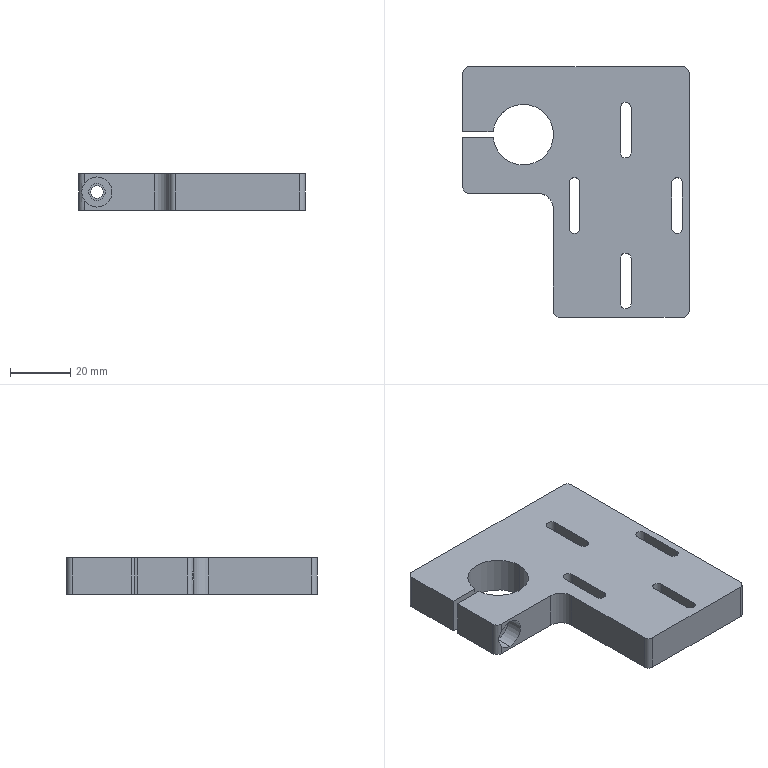Part | SolidWorks | features ICE 4, HoleWzd 3, Fillet 2, LPattern 2, Extrusion 1, MoveFace 1 | 1 solid | 42 faces | box 75 x 83 x 12 mm | volume 51875 mm3 | cylinder 22 | plane 20 | commonest cylinder face diameters 3.5 x8 4 x5 10 x3 4.2 x2 5.5 x2 20.1 x2
STEP:
#1=CARTESIAN_POINT('',(-31.5,40.,2.1));
#2=VERTEX_POINT('',#1);
#3=CARTESIAN_POINT('',(-31.5,40.,-2.1));
#4=VERTEX_POINT('',#3);
#5=CARTESIAN_POINT('',(-31.5,40.,0.));
#6=DIRECTION('',(0.,-1.,0.));
#7=DIRECTION('',(1.,0.,0.));
#8=AXIS2_PLACEMENT_3D('',#5,#6,#7);
#9=CIRCLE('',#8,2.1);
#10=EDGE_CURVE('',#2,#4,#9,.T.);
#11=ORIENTED_EDGE('',*,*,#10,.F.);
#12=CARTESIAN_POINT('',(-31.5,18.5,2.1));
#13=VERTEX_POINT('',#12);
#14=CARTESIAN_POINT('',(-31.5,18.5,2.1));
#15=DIRECTION('',(0.,-1.,0.));
#16=VECTOR('',#15,1000.);
#17=LINE('',#14,#16);
#18=EDGE_CURVE('',#2,#13,#17,.T.);
#19=ORIENTED_EDGE('',*,*,#18,.T.);
#20=CARTESIAN_POINT('',(-31.5,18.5,-2.1));
#21=VERTEX_POINT('',#20);
#22=CARTESIAN_POINT('',(-31.5,18.5,0.));
#23=DIRECTION('',(0.,-1.,0.));
#24=DIRECTION('',(0.,0.,-1.));
#25=AXIS2_PLACEMENT_3D('',#22,#23,#24);
#26=CIRCLE('',#25,2.1);
#27=EDGE_CURVE('',#13,#21,#26,.T.);
#28=ORIENTED_EDGE('',*,*,#27,.T.);
#29=CARTESIAN_POINT('',(-31.5,18.5,-2.1));
#30=DIRECTION('',(0.,-1.,0.));
#31=VECTOR('',#30,1000.);
#32=LINE('',#29,#31);
#33=EDGE_CURVE('',#4,#21,#32,.T.);
#34=ORIENTED_EDGE('',*,*,#33,.F.);
#35=EDGE_LOOP('',(#11,#19,#28,#34));
#36=FACE_OUTER_BOUND('',#35,.T.);
#37=CARTESIAN_POINT('',(-31.5,18.5,0.));
#38=DIRECTION('',(0.,-1.,0.));
#39=DIRECTION('',(0.,0.,-1.));
#40=AXIS2_PLACEMENT_3D('',#37,#38,#39);
#41=CYLINDRICAL_SURFACE('',#40,2.1);
#42=ADVANCED_FACE('',(#36),#41,.F.);
#43=CARTESIAN_POINT('',(-31.5,3.7,5.));
#44=VERTEX_POINT('',#43);
#45=CARTESIAN_POINT('',(-31.5,3.7,-5.));
#46=VERTEX_POINT('',#45);
#47=CARTESIAN_POINT('',(-31.5,3.7,0.));
#48=DIRECTION('',(0.,-1.,0.));
#49=DIRECTION('',(0.,0.,-1.));
#50=AXIS2_PLACEMENT_3D('',#47,#48,#49);
#51=CIRCLE('',#50,5.);
#52=EDGE_CURVE('',#44,#46,#51,.T.);
#53=ORIENTED_EDGE('',*,*,#52,.F.);
#54=CARTESIAN_POINT('',(-31.5,-2.,5.));
#55=VERTEX_POINT('',#54);
#56=CARTESIAN_POINT('',(-31.5,-2.,5.));
#57=DIRECTION('',(0.,-1.,0.));
#58=VECTOR('',#57,1000.);
#59=LINE('',#56,#58);
#60=EDGE_CURVE('',#44,#55,#59,.T.);
#61=ORIENTED_EDGE('',*,*,#60,.T.);
#62=CARTESIAN_POINT('',(-35.5,-2.,3.));
#63=VERTEX_POINT('',#62);
#64=CARTESIAN_POINT('',(-31.5,-2.,0.));
#65=DIRECTION('',(0.,-1.,0.));
#66=DIRECTION('',(0.,0.,-1.));
#67=AXIS2_PLACEMENT_3D('',#64,#65,#66);
#68=CIRCLE('',#67,5.);
#69=EDGE_CURVE('',#55,#63,#68,.T.);
#70=ORIENTED_EDGE('',*,*,#69,.T.);
#71=CARTESIAN_POINT('',(-35.5,-2.,-3.));
#72=VERTEX_POINT('',#71);
#73=CARTESIAN_POINT('',(-35.5,-2.,3.));
#74=CARTESIAN_POINT('',(-35.663,-2.,2.782));
#75=CARTESIAN_POINT('',(-35.806,-1.981,2.555));
#76=CARTESIAN_POINT('',(-36.054,-1.926,2.082));
#77=CARTESIAN_POINT('',(-36.159,-1.891,1.835));
#78=CARTESIAN_POINT('',(-36.328,-1.823,1.326));
#79=CARTESIAN_POINT('',(-36.392,-1.791,1.067));
#80=CARTESIAN_POINT('',(-36.478,-1.745,0.5398));
#81=CARTESIAN_POINT('',(-36.5,-1.732,0.2681));
#82=CARTESIAN_POINT('',(-36.5,-1.732,-0.271));
#83=CARTESIAN_POINT('',(-36.478,-1.745,-0.5373));
#84=CARTESIAN_POINT('',(-36.393,-1.79,-1.064));
#85=CARTESIAN_POINT('',(-36.328,-1.823,-1.326));
#86=CARTESIAN_POINT('',(-36.159,-1.89,-1.834));
#87=CARTESIAN_POINT('',(-36.055,-1.926,-2.079));
#88=CARTESIAN_POINT('',(-35.808,-1.98,-2.552));
#89=CARTESIAN_POINT('',(-35.663,-2.,-2.783));
#90=CARTESIAN_POINT('',(-35.5,-2.,-3.));
#91=B_SPLINE_CURVE_WITH_KNOTS('',3,(#73,#74,#75,#76,#77,#78,#79,#80,#81,#82,#83,#84,#85,#86,#87,#88,#89,#90),.UNSPECIFIED.,.F.,.F.,(4,2,2,2,2,2,2,2,4),(0.,0.0008047,0.001609,0.002414,0.003219,0.004024,0.004828,0.005633,0.006438),.UNSPECIFIED.);
#92=EDGE_CURVE('',#63,#72,#91,.T.);
#93=ORIENTED_EDGE('',*,*,#92,.T.);
#94=CARTESIAN_POINT('',(-31.5,-2.,-5.));
#95=VERTEX_POINT('',#94);
#96=CARTESIAN_POINT('',(-31.5,-2.,0.));
#97=DIRECTION('',(0.,-1.,0.));
#98=DIRECTION('',(0.,0.,-1.));
#99=AXIS2_PLACEMENT_3D('',#96,#97,#98);
#100=CIRCLE('',#99,5.);
#101=EDGE_CURVE('',#72,#95,#100,.T.);
#102=ORIENTED_EDGE('',*,*,#101,.T.);
#103=CARTESIAN_POINT('',(-31.5,-2.,-5.));
#104=DIRECTION('',(0.,-1.,0.));
#105=VECTOR('',#104,1000.);
#106=LINE('',#103,#105);
#107=EDGE_CURVE('',#46,#95,#106,.T.);
#108=ORIENTED_EDGE('',*,*,#107,.F.);
#109=EDGE_LOOP('',(#53,#61,#70,#93,#102,#108));
#110=FACE_OUTER_BOUND('',#109,.T.);
#111=CARTESIAN_POINT('',(-31.5,-2.,0.));
#112=DIRECTION('',(0.,-1.,0.));
#113=DIRECTION('',(0.,0.,-1.));
#114=AXIS2_PLACEMENT_3D('',#111,#112,#113);
#115=CYLINDRICAL_SURFACE('',#114,5.);
#116=ADVANCED_FACE('',(#110),#115,.F.);
#117=CARTESIAN_POINT('',(-31.5,16.5,2.75));
#118=VERTEX_POINT('',#117);
#119=CARTESIAN_POINT('',(-31.5,16.5,-2.75));
#120=VERTEX_POINT('',#119);
#121=CARTESIAN_POINT('',(-31.5,16.5,0.));
#122=DIRECTION('',(0.,-1.,0.));
#123=DIRECTION('',(1.,0.,0.));
#124=AXIS2_PLACEMENT_3D('',#121,#122,#123);
#125=CIRCLE('',#124,2.75);
#126=EDGE_CURVE('',#118,#120,#125,.T.);
#127=ORIENTED_EDGE('',*,*,#126,.F.);
#128=CARTESIAN_POINT('',(-31.5,3.7,2.75));
#129=VERTEX_POINT('',#128);
#130=CARTESIAN_POINT('',(-31.5,-2.,2.75));
#131=DIRECTION('',(0.,-1.,0.));
#132=VECTOR('',#131,1000.);
#133=LINE('',#130,#132);
#134=EDGE_CURVE('',#118,#129,#133,.T.);
#135=ORIENTED_EDGE('',*,*,#134,.T.);
#136=CARTESIAN_POINT('',(-31.5,3.7,-2.75));
#137=VERTEX_POINT('',#136);
#138=CARTESIAN_POINT('',(-31.5,3.7,0.));
#139=DIRECTION('',(0.,-1.,0.));
#140=DIRECTION('',(0.,0.,-1.));
#141=AXIS2_PLACEMENT_3D('',#138,#139,#140);
#142=CIRCLE('',#141,2.75);
#143=EDGE_CURVE('',#129,#137,#142,.T.);
#144=ORIENTED_EDGE('',*,*,#143,.T.);
#145=CARTESIAN_POINT('',(-31.5,-2.,-2.75));
#146=DIRECTION('',(0.,-1.,0.));
#147=VECTOR('',#146,1000.);
#148=LINE('',#145,#147);
#149=EDGE_CURVE('',#120,#137,#148,.T.);
#150=ORIENTED_EDGE('',*,*,#149,.F.);
#151=EDGE_LOOP('',(#127,#135,#144,#150));
#152=FACE_OUTER_BOUND('',#151,.T.);
#153=CARTESIAN_POINT('',(-31.5,-2.,0.));
#154=DIRECTION('',(0.,-1.,0.));
#155=DIRECTION('',(0.,0.,-1.));
#156=AXIS2_PLACEMENT_3D('',#153,#154,#155);
#157=CYLINDRICAL_SURFACE('',#156,2.75);
#158=ADVANCED_FACE('',(#152),#157,.F.);
#159=CARTESIAN_POINT('',(-27.5,18.5,-6.));
#160=VERTEX_POINT('',#159);
#161=CARTESIAN_POINT('',(-7.45,17.5,-6.));
#162=VERTEX_POINT('',#161);
#163=CARTESIAN_POINT('',(-17.5,17.5,-6.));
#164=DIRECTION('',(0.,0.,-1.));
#165=DIRECTION('',(1.,0.,0.));
#166=AXIS2_PLACEMENT_3D('',#163,#164,#165);
#167=CIRCLE('',#166,10.05);
#168=EDGE_CURVE('',#160,#162,#167,.T.);
#169=ORIENTED_EDGE('',*,*,#168,.T.);
#170=CARTESIAN_POINT('',(-7.45,17.5,6.));
#171=VERTEX_POINT('',#170);
#172=CARTESIAN_POINT('',(-7.45,17.5,-6.001));
#173=DIRECTION('',(0.,0.,1.));
#174=VECTOR('',#173,1000.);
#175=LINE('',#172,#174);
#176=EDGE_CURVE('',#162,#171,#175,.T.);
#177=ORIENTED_EDGE('',*,*,#176,.T.);
#178=CARTESIAN_POINT('',(-27.5,18.5,6.));
#179=VERTEX_POINT('',#178);
#180=CARTESIAN_POINT('',(-17.5,17.5,6.));
#181=DIRECTION('',(0.,0.,1.));
#182=DIRECTION('',(1.,0.,0.));
#183=AXIS2_PLACEMENT_3D('',#180,#181,#182);
#184=CIRCLE('',#183,10.05);
#185=EDGE_CURVE('',#171,#179,#184,.T.);
#186=ORIENTED_EDGE('',*,*,#185,.T.);
#187=CARTESIAN_POINT('',(-27.5,18.5,-6.001));
#188=DIRECTION('',(0.,0.,1.));
#189=VECTOR('',#188,1000.);
#190=LINE('',#187,#189);
#191=EDGE_CURVE('',#160,#179,#190,.T.);
#192=ORIENTED_EDGE('',*,*,#191,.F.);
#193=EDGE_LOOP('',(#169,#177,#186,#192));
#194=FACE_OUTER_BOUND('',#193,.T.);
#195=CARTESIAN_POINT('',(-17.5,17.5,-6.001));
#196=DIRECTION('',(0.,0.,1.));
#197=DIRECTION('',(1.,0.,0.));
#198=AXIS2_PLACEMENT_3D('',#195,#196,#197);
#199=CYLINDRICAL_SURFACE('',#198,10.05);
#200=ADVANCED_FACE('',(#194),#199,.F.);
#201=ORIENTED_EDGE('',*,*,#101,.F.);
#202=CARTESIAN_POINT('',(-35.5,-2.,-6.));
#203=VERTEX_POINT('',#202);
#204=CARTESIAN_POINT('',(-35.5,-2.,6.001));
#205=DIRECTION('',(0.,0.,-1.));
#206=VECTOR('',#205,1000.);
#207=LINE('',#204,#206);
#208=EDGE_CURVE('',#72,#203,#207,.T.);
#209=ORIENTED_EDGE('',*,*,#208,.T.);
#210=CARTESIAN_POINT('',(-12.5,-2.,-6.));
#211=VERTEX_POINT('',#210);
#212=CARTESIAN_POINT('',(-37.5,-2.,-6.));
#213=DIRECTION('',(1.,0.,0.));
#214=VECTOR('',#213,1000.);
#215=LINE('',#212,#214);
#216=EDGE_CURVE('',#203,#211,#215,.T.);
#217=ORIENTED_EDGE('',*,*,#216,.T.);
#218=CARTESIAN_POINT('',(-12.5,-2.,6.));
#219=VERTEX_POINT('',#218);
#220=CARTESIAN_POINT('',(-12.5,-2.,6.));
#221=DIRECTION('',(0.,0.,1.));
#222=VECTOR('',#221,1000.);
#223=LINE('',#220,#222);
#224=EDGE_CURVE('',#211,#219,#223,.T.);
#225=ORIENTED_EDGE('',*,*,#224,.T.);
#226=CARTESIAN_POINT('',(-35.5,-2.,6.));
#227=VERTEX_POINT('',#226);
#228=CARTESIAN_POINT('',(-37.5,-2.,6.));
#229=DIRECTION('',(1.,0.,0.));
#230=VECTOR('',#229,1000.);
#231=LINE('',#228,#230);
#232=EDGE_CURVE('',#227,#219,#231,.T.);
#233=ORIENTED_EDGE('',*,*,#232,.F.);
#234=CARTESIAN_POINT('',(-35.5,-2.,6.001));
#235=DIRECTION('',(0.,0.,-1.));
#236=VECTOR('',#235,1000.);
#237=LINE('',#234,#236);
#238=EDGE_CURVE('',#227,#63,#237,.T.);
#239=ORIENTED_EDGE('',*,*,#238,.T.);
#240=ORIENTED_EDGE('',*,*,#69,.F.);
#241=CARTESIAN_POINT('',(-31.5,-2.,0.));
#242=DIRECTION('',(0.,-1.,0.));
#243=DIRECTION('',(0.,0.,-1.));
#244=AXIS2_PLACEMENT_3D('',#241,#242,#243);
#245=CIRCLE('',#244,5.);
#246=EDGE_CURVE('',#95,#55,#245,.T.);
#247=ORIENTED_EDGE('',*,*,#246,.F.);
#248=EDGE_LOOP('',(#201,#209,#217,#225,#233,#239,#240,#247));
#249=FACE_OUTER_BOUND('',#248,.T.);
#250=CARTESIAN_POINT('',(-37.5,-2.,6.001));
#251=DIRECTION('',(0.,1.,0.));
#252=DIRECTION('',(-1.,0.,0.));
#253=AXIS2_PLACEMENT_3D('',#250,#251,#252);
#254=PLANE('',#253);
#255=ADVANCED_FACE('',(#249),#254,.F.);
#256=CARTESIAN_POINT('',(31.75,-13.5,-6.));
#257=VERTEX_POINT('',#256);
#258=CARTESIAN_POINT('',(31.75,1.5,-6.));
#259=VERTEX_POINT('',#258);
#260=CARTESIAN_POINT('',(31.75,-13.5,-6.));
#261=DIRECTION('',(0.,1.,0.));
#262=VECTOR('',#261,1000.);
#263=LINE('',#260,#262);
#264=EDGE_CURVE('',#257,#259,#263,.T.);
#265=ORIENTED_EDGE('',*,*,#264,.F.);
#266=CARTESIAN_POINT('',(35.25,-13.5,-6.));
#267=VERTEX_POINT('',#266);
#268=CARTESIAN_POINT('',(33.5,-13.5,-6.));
#269=DIRECTION('',(0.,0.,-1.));
#270=DIRECTION('',(-1.,0.,0.));
#271=AXIS2_PLACEMENT_3D('',#268,#269,#270);
#272=CIRCLE('',#271,1.75);
#273=EDGE_CURVE('',#267,#257,#272,.T.);
#274=ORIENTED_EDGE('',*,*,#273,.F.);
#275=CARTESIAN_POINT('',(35.25,1.5,-6.));
#276=VERTEX_POINT('',#275);
#277=CARTESIAN_POINT('',(35.25,-13.5,-6.));
#278=DIRECTION('',(0.,-1.,0.));
#279=VECTOR('',#278,1000.);
#280=LINE('',#277,#279);
#281=EDGE_CURVE('',#276,#267,#280,.T.);
#282=ORIENTED_EDGE('',*,*,#281,.F.);
#283=CARTESIAN_POINT('',(33.5,1.5,-6.));
#284=DIRECTION('',(0.,0.,-1.));
#285=DIRECTION('',(-1.,0.,0.));
#286=AXIS2_PLACEMENT_3D('',#283,#284,#285);
#287=CIRCLE('',#286,1.75);
#288=EDGE_CURVE('',#259,#276,#287,.T.);
#289=ORIENTED_EDGE('',*,*,#288,.F.);
#290=EDGE_LOOP('',(#265,#274,#282,#289));
#291=FACE_BOUND('',#290,.T.);
#292=CARTESIAN_POINT('',(14.75,-38.5,-6.));
#293=VERTEX_POINT('',#292);
#294=CARTESIAN_POINT('',(14.75,-23.5,-6.));
#295=VERTEX_POINT('',#294);
#296=CARTESIAN_POINT('',(14.75,-38.5,-6.));
#297=DIRECTION('',(0.,1.,0.));
#298=VECTOR('',#297,1000.);
#299=LINE('',#296,#298);
#300=EDGE_CURVE('',#293,#295,#299,.T.);
#301=ORIENTED_EDGE('',*,*,#300,.F.);
#302=CARTESIAN_POINT('',(18.25,-38.5,-6.));
#303=VERTEX_POINT('',#302);
#304=CARTESIAN_POINT('',(16.5,-38.5,-6.));
#305=DIRECTION('',(0.,0.,-1.));
#306=DIRECTION('',(-1.,0.,0.));
#307=AXIS2_PLACEMENT_3D('',#304,#305,#306);
#308=CIRCLE('',#307,1.75);
#309=EDGE_CURVE('',#303,#293,#308,.T.);
#310=ORIENTED_EDGE('',*,*,#309,.F.);
#311=CARTESIAN_POINT('',(18.25,-23.5,-6.));
#312=VERTEX_POINT('',#311);
#313=CARTESIAN_POINT('',(18.25,-38.5,-6.));
#314=DIRECTION('',(0.,-1.,0.));
#315=VECTOR('',#314,1000.);
#316=LINE('',#313,#315);
#317=EDGE_CURVE('',#312,#303,#316,.T.);
#318=ORIENTED_EDGE('',*,*,#317,.F.);
#319=CARTESIAN_POINT('',(16.5,-23.5,-6.));
#320=DIRECTION('',(0.,0.,-1.));
#321=DIRECTION('',(-1.,0.,0.));
#322=AXIS2_PLACEMENT_3D('',#319,#320,#321);
#323=CIRCLE('',#322,1.75);
#324=EDGE_CURVE('',#295,#312,#323,.T.);
#325=ORIENTED_EDGE('',*,*,#324,.F.);
#326=EDGE_LOOP('',(#301,#310,#318,#325));
#327=FACE_BOUND('',#326,.T.);
#328=CARTESIAN_POINT('',(-2.25,-13.5,-6.));
#329=VERTEX_POINT('',#328);
#330=CARTESIAN_POINT('',(-2.25,1.5,-6.));
#331=VERTEX_POINT('',#330);
#332=CARTESIAN_POINT('',(-2.25,-13.5,-6.));
#333=DIRECTION('',(0.,1.,0.));
#334=VECTOR('',#333,1000.);
#335=LINE('',#332,#334);
#336=EDGE_CURVE('',#329,#331,#335,.T.);
#337=ORIENTED_EDGE('',*,*,#336,.F.);
#338=CARTESIAN_POINT('',(1.25,-13.5,-6.));
#339=VERTEX_POINT('',#338);
#340=CARTESIAN_POINT('',(-0.5,-13.5,-6.));
#341=DIRECTION('',(0.,0.,-1.));
#342=DIRECTION('',(-1.,0.,0.));
#343=AXIS2_PLACEMENT_3D('',#340,#341,#342);
#344=CIRCLE('',#343,1.75);
#345=EDGE_CURVE('',#339,#329,#344,.T.);
#346=ORIENTED_EDGE('',*,*,#345,.F.);
#347=CARTESIAN_POINT('',(1.25,1.5,-6.));
#348=VERTEX_POINT('',#347);
#349=CARTESIAN_POINT('',(1.25,-13.5,-6.));
#350=DIRECTION('',(0.,-1.,0.));
#351=VECTOR('',#350,1000.);
#352=LINE('',#349,#351);
#353=EDGE_CURVE('',#348,#339,#352,.T.);
#354=ORIENTED_EDGE('',*,*,#353,.F.);
#355=CARTESIAN_POINT('',(-0.5,1.5,-6.));
#356=DIRECTION('',(0.,0.,-1.));
#357=DIRECTION('',(-1.,0.,0.));
#358=AXIS2_PLACEMENT_3D('',#355,#356,#357);
#359=CIRCLE('',#358,1.75);
#360=EDGE_CURVE('',#331,#348,#359,.T.);
#361=ORIENTED_EDGE('',*,*,#360,.F.);
#362=EDGE_LOOP('',(#337,#346,#354,#361));
#363=FACE_BOUND('',#362,.T.);
#364=CARTESIAN_POINT('',(14.75,11.5,-6.));
#365=VERTEX_POINT('',#364);
#366=CARTESIAN_POINT('',(14.75,26.5,-6.));
#367=VERTEX_POINT('',#366);
#368=CARTESIAN_POINT('',(14.75,11.5,-6.));
#369=DIRECTION('',(0.,1.,0.));
#370=VECTOR('',#369,1000.);
#371=LINE('',#368,#370);
#372=EDGE_CURVE('',#365,#367,#371,.T.);
#373=ORIENTED_EDGE('',*,*,#372,.F.);
#374=CARTESIAN_POINT('',(18.25,11.5,-6.));
#375=VERTEX_POINT('',#374);
#376=CARTESIAN_POINT('',(16.5,11.5,-6.));
#377=DIRECTION('',(0.,0.,-1.));
#378=DIRECTION('',(-1.,0.,0.));
#379=AXIS2_PLACEMENT_3D('',#376,#377,#378);
#380=CIRCLE('',#379,1.75);
#381=EDGE_CURVE('',#375,#365,#380,.T.);
#382=ORIENTED_EDGE('',*,*,#381,.F.);
#383=CARTESIAN_POINT('',(18.25,26.5,-6.));
#384=VERTEX_POINT('',#383);
#385=CARTESIAN_POINT('',(18.25,11.5,-6.));
#386=DIRECTION('',(0.,-1.,0.));
#387=VECTOR('',#386,1000.);
#388=LINE('',#385,#387);
#389=EDGE_CURVE('',#384,#375,#388,.T.);
#390=ORIENTED_EDGE('',*,*,#389,.F.);
#391=CARTESIAN_POINT('',(16.5,26.5,-6.));
#392=DIRECTION('',(0.,0.,-1.));
#393=DIRECTION('',(-1.,0.,0.));
#394=AXIS2_PLACEMENT_3D('',#391,#392,#393);
#395=CIRCLE('',#394,1.75);
#396=EDGE_CURVE('',#367,#384,#395,.T.);
#397=ORIENTED_EDGE('',*,*,#396,.F.);
#398=EDGE_LOOP('',(#373,#382,#390,#397));
#399=FACE_BOUND('',#398,.T.);
#400=CARTESIAN_POINT('',(35.5,40.,-6.));
#401=VERTEX_POINT('',#400);
#402=CARTESIAN_POINT('',(-35.5,40.,-6.));
#403=VERTEX_POINT('',#402);
#404=CARTESIAN_POINT('',(37.5,40.,-6.));
#405=DIRECTION('',(-1.,0.,0.));
#406=VECTOR('',#405,1000.);
#407=LINE('',#404,#406);
#408=EDGE_CURVE('',#401,#403,#407,.T.);
#409=ORIENTED_EDGE('',*,*,#408,.F.);
#410=CARTESIAN_POINT('',(37.5,38.,-6.));
#411=VERTEX_POINT('',#410);
#412=CARTESIAN_POINT('',(35.5,38.,-6.));
#413=DIRECTION('',(0.,0.,-1.));
#414=DIRECTION('',(1.,0.,0.));
#415=AXIS2_PLACEMENT_3D('',#412,#413,#414);
#416=CIRCLE('',#415,2.);
#417=EDGE_CURVE('',#401,#411,#416,.T.);
#418=ORIENTED_EDGE('',*,*,#417,.T.);
#419=CARTESIAN_POINT('',(37.5,-41.,-6.));
#420=VERTEX_POINT('',#419);
#421=CARTESIAN_POINT('',(37.5,-40.,-6.));
#422=DIRECTION('',(0.,1.,0.));
#423=VECTOR('',#422,1000.);
#424=LINE('',#421,#423);
#425=EDGE_CURVE('',#420,#411,#424,.T.);
#426=ORIENTED_EDGE('',*,*,#425,.F.);
#427=CARTESIAN_POINT('',(35.5,-43.,-6.));
#428=VERTEX_POINT('',#427);
#429=CARTESIAN_POINT('',(35.5,-41.,-6.));
#430=DIRECTION('',(0.,0.,-1.));
#431=DIRECTION('',(1.,0.,0.));
#432=AXIS2_PLACEMENT_3D('',#429,#430,#431);
#433=CIRCLE('',#432,2.);
#434=EDGE_CURVE('',#420,#428,#433,.T.);
#435=ORIENTED_EDGE('',*,*,#434,.T.);
#436=CARTESIAN_POINT('',(-5.5,-43.,-6.));
#437=VERTEX_POINT('',#436);
#438=CARTESIAN_POINT('',(37.5,-43.,-6.));
#439=DIRECTION('',(1.,0.,0.));
#440=VECTOR('',#439,1000.);
#441=LINE('',#438,#440);
#442=EDGE_CURVE('',#437,#428,#441,.T.);
#443=ORIENTED_EDGE('',*,*,#442,.F.);
#444=CARTESIAN_POINT('',(-7.5,-41.,-6.));
#445=VERTEX_POINT('',#444);
#446=CARTESIAN_POINT('',(-5.5,-41.,-6.));
#447=DIRECTION('',(0.,0.,-1.));
#448=DIRECTION('',(1.,0.,0.));
#449=AXIS2_PLACEMENT_3D('',#446,#447,#448);
#450=CIRCLE('',#449,2.);
#451=EDGE_CURVE('',#437,#445,#450,.T.);
#452=ORIENTED_EDGE('',*,*,#451,.T.);
#453=CARTESIAN_POINT('',(-7.5,-7.,-6.));
#454=VERTEX_POINT('',#453);
#455=CARTESIAN_POINT('',(-7.5,-2.,-6.));
#456=DIRECTION('',(0.,-1.,0.));
#457=VECTOR('',#456,1000.);
#458=LINE('',#455,#457);
#459=EDGE_CURVE('',#454,#445,#458,.T.);
#460=ORIENTED_EDGE('',*,*,#459,.F.);
#461=CARTESIAN_POINT('',(-12.5,-7.,-6.));
#462=DIRECTION('',(0.,0.,1.));
#463=DIRECTION('',(1.,0.,0.));
#464=AXIS2_PLACEMENT_3D('',#461,#462,#463);
#465=CIRCLE('',#464,5.);
#466=EDGE_CURVE('',#454,#211,#465,.T.);
#467=ORIENTED_EDGE('',*,*,#466,.T.);
#468=ORIENTED_EDGE('',*,*,#216,.F.);
#469=CARTESIAN_POINT('',(-37.5,0.,-6.));
#470=VERTEX_POINT('',#469);
#471=CARTESIAN_POINT('',(-35.5,0.,-6.));
#472=DIRECTION('',(0.,0.,-1.));
#473=DIRECTION('',(1.,0.,0.));
#474=AXIS2_PLACEMENT_3D('',#471,#472,#473);
#475=CIRCLE('',#474,2.);
#476=EDGE_CURVE('',#203,#470,#475,.T.);
#477=ORIENTED_EDGE('',*,*,#476,.T.);
#478=CARTESIAN_POINT('',(-37.5,16.5,-6.));
#479=VERTEX_POINT('',#478);
#480=CARTESIAN_POINT('',(-37.5,-40.,-6.));
#481=DIRECTION('',(0.,-1.,0.));
#482=VECTOR('',#481,1000.);
#483=LINE('',#480,#482);
#484=EDGE_CURVE('',#479,#470,#483,.T.);
#485=ORIENTED_EDGE('',*,*,#484,.F.);
#486=CARTESIAN_POINT('',(-27.5,16.5,-6.));
#487=VERTEX_POINT('',#486);
#488=CARTESIAN_POINT('',(-52.59,16.5,-6.));
#489=DIRECTION('',(-1.,0.,0.));
#490=VECTOR('',#489,1000.);
#491=LINE('',#488,#490);
#492=EDGE_CURVE('',#487,#479,#491,.T.);
#493=ORIENTED_EDGE('',*,*,#492,.F.);
#494=CARTESIAN_POINT('',(-17.5,17.5,-6.));
#495=DIRECTION('',(0.,0.,-1.));
#496=DIRECTION('',(1.,0.,0.));
#497=AXIS2_PLACEMENT_3D('',#494,#495,#496);
#498=CIRCLE('',#497,10.05);
#499=EDGE_CURVE('',#162,#487,#498,.T.);
#500=ORIENTED_EDGE('',*,*,#499,.F.);
#501=ORIENTED_EDGE('',*,*,#168,.F.);
#502=CARTESIAN_POINT('',(-37.5,18.5,-6.));
#503=VERTEX_POINT('',#502);
#504=CARTESIAN_POINT('',(-52.59,18.5,-6.));
#505=DIRECTION('',(1.,0.,0.));
#506=VECTOR('',#505,1000.);
#507=LINE('',#504,#506);
#508=EDGE_CURVE('',#503,#160,#507,.T.);
#509=ORIENTED_EDGE('',*,*,#508,.F.);
#510=CARTESIAN_POINT('',(-37.5,38.,-6.));
#511=VERTEX_POINT('',#510);
#512=CARTESIAN_POINT('',(-37.5,-40.,-6.));
#513=DIRECTION('',(0.,-1.,0.));
#514=VECTOR('',#513,1000.);
#515=LINE('',#512,#514);
#516=EDGE_CURVE('',#511,#503,#515,.T.);
#517=ORIENTED_EDGE('',*,*,#516,.F.);
#518=CARTESIAN_POINT('',(-35.5,38.,-6.));
#519=DIRECTION('',(0.,0.,-1.));
#520=DIRECTION('',(1.,0.,0.));
#521=AXIS2_PLACEMENT_3D('',#518,#519,#520);
#522=CIRCLE('',#521,2.);
#523=EDGE_CURVE('',#511,#403,#522,.T.);
#524=ORIENTED_EDGE('',*,*,#523,.T.);
#525=EDGE_LOOP('',(#409,#418,#426,#435,#443,#452,#460,#467,#468,#477,#485,#493,#500,#501,#509,#517,#524));
#526=FACE_OUTER_BOUND('',#525,.T.);
#527=CARTESIAN_POINT('',(0.,0.,-6.));
#528=DIRECTION('',(0.,0.,1.));
#529=DIRECTION('',(1.,0.,0.));
#530=AXIS2_PLACEMENT_3D('',#527,#528,#529);
#531=PLANE('',#530);
#532=ADVANCED_FACE('',(#291,#327,#363,#399,#526),#531,.F.);
#533=CARTESIAN_POINT('',(-37.5,38.,6.));
#534=VERTEX_POINT('',#533);
#535=CARTESIAN_POINT('',(-37.5,18.5,6.));
#536=VERTEX_POINT('',#535);
#537=CARTESIAN_POINT('',(-37.5,-40.,6.));
#538=DIRECTION('',(0.,-1.,0.));
#539=VECTOR('',#538,1000.);
#540=LINE('',#537,#539);
#541=EDGE_CURVE('',#534,#536,#540,.T.);
#542=ORIENTED_EDGE('',*,*,#541,.F.);
#543=CARTESIAN_POINT('',(-37.5,38.,6.));
#544=DIRECTION('',(0.,0.,-1.));
#545=VECTOR('',#544,1000.);
#546=LINE('',#543,#545);
#547=EDGE_CURVE('',#534,#511,#546,.T.);
#548=ORIENTED_EDGE('',*,*,#547,.T.);
#549=ORIENTED_EDGE('',*,*,#516,.T.);
#550=CARTESIAN_POINT('',(-37.5,18.5,6.001));
#551=DIRECTION('',(0.,0.,-1.));
#552=VECTOR('',#551,1000.);
#553=LINE('',#550,#552);
#554=EDGE_CURVE('',#536,#503,#553,.T.);
#555=ORIENTED_EDGE('',*,*,#554,.F.);
#556=EDGE_LOOP('',(#542,#548,#549,#555));
#557=FACE_OUTER_BOUND('',#556,.T.);
#558=CARTESIAN_POINT('',(-37.5,-40.,6.));
#559=DIRECTION('',(1.,0.,0.));
#560=DIRECTION('',(0.,0.,-1.));
#561=AXIS2_PLACEMENT_3D('',#558,#559,#560);
#562=PLANE('',#561);
#563=ADVANCED_FACE('',(#557),#562,.F.);
#564=ORIENTED_EDGE('',*,*,#484,.T.);
#565=CARTESIAN_POINT('',(-37.5,0.,6.));
#566=VERTEX_POINT('',#565);
#567=CARTESIAN_POINT('',(-37.5,0.,6.));
#568=DIRECTION('',(0.,0.,1.));
#569=VECTOR('',#568,1000.);
#570=LINE('',#567,#569);
#571=EDGE_CURVE('',#470,#566,#570,.T.);
#572=ORIENTED_EDGE('',*,*,#571,.T.);
#573=CARTESIAN_POINT('',(-37.5,16.5,6.));
#574=VERTEX_POINT('',#573);
#575=CARTESIAN_POINT('',(-37.5,-40.,6.));
#576=DIRECTION('',(0.,-1.,0.));
#577=VECTOR('',#576,1000.);
#578=LINE('',#575,#577);
#579=EDGE_CURVE('',#574,#566,#578,.T.);
#580=ORIENTED_EDGE('',*,*,#579,.F.);
#581=CARTESIAN_POINT('',(-37.5,16.5,6.001));
#582=DIRECTION('',(0.,0.,1.));
#583=VECTOR('',#582,1000.);
#584=LINE('',#581,#583);
#585=EDGE_CURVE('',#479,#574,#584,.T.);
#586=ORIENTED_EDGE('',*,*,#585,.F.);
#587=EDGE_LOOP('',(#564,#572,#580,#586));
#588=FACE_OUTER_BOUND('',#587,.T.);
#589=CARTESIAN_POINT('',(-37.5,-40.,6.));
#590=DIRECTION('',(1.,0.,0.));
#591=DIRECTION('',(0.,0.,-1.));
#592=AXIS2_PLACEMENT_3D('',#589,#590,#591);
#593=PLANE('',#592);
#594=ADVANCED_FACE('',(#588),#593,.F.);
#595=ORIENTED_EDGE('',*,*,#442,.T.);
#596=CARTESIAN_POINT('',(35.5,-43.,6.));
#597=VERTEX_POINT('',#596);
#598=CARTESIAN_POINT('',(35.5,-43.,6.));
#599=DIRECTION('',(0.,0.,1.));
#600=VECTOR('',#599,1000.);
#601=LINE('',#598,#600);
#602=EDGE_CURVE('',#428,#597,#601,.T.);
#603=ORIENTED_EDGE('',*,*,#602,.T.);
#604=CARTESIAN_POINT('',(-5.5,-43.,6.));
#605=VERTEX_POINT('',#604);
#606=CARTESIAN_POINT('',(37.5,-43.,6.));
#607=DIRECTION('',(1.,0.,0.));
#608=VECTOR('',#607,1000.);
#609=LINE('',#606,#608);
#610=EDGE_CURVE('',#605,#597,#609,.T.);
#611=ORIENTED_EDGE('',*,*,#610,.F.);
#612=CARTESIAN_POINT('',(-5.5,-43.,6.));
#613=DIRECTION('',(0.,0.,-1.));
#614=VECTOR('',#613,1000.);
#615=LINE('',#612,#614);
#616=EDGE_CURVE('',#605,#437,#615,.T.);
#617=ORIENTED_EDGE('',*,*,#616,.T.);
#618=EDGE_LOOP('',(#595,#603,#611,#617));
#619=FACE_OUTER_BOUND('',#618,.T.);
#620=CARTESIAN_POINT('',(37.5,-43.,6.));
#621=DIRECTION('',(0.,1.,0.));
#622=DIRECTION('',(-1.,0.,0.));
#623=AXIS2_PLACEMENT_3D('',#620,#621,#622);
#624=PLANE('',#623);
#625=ADVANCED_FACE('',(#619),#624,.F.);
#626=ORIENTED_EDGE('',*,*,#425,.T.);
#627=CARTESIAN_POINT('',(37.5,38.,6.));
#628=VERTEX_POINT('',#627);
#629=CARTESIAN_POINT('',(37.5,38.,6.));
#630=DIRECTION('',(0.,0.,1.));
#631=VECTOR('',#630,1000.);
#632=LINE('',#629,#631);
#633=EDGE_CURVE('',#411,#628,#632,.T.);
#634=ORIENTED_EDGE('',*,*,#633,.T.);
#635=CARTESIAN_POINT('',(37.5,-41.,6.));
#636=VERTEX_POINT('',#635);
#637=CARTESIAN_POINT('',(37.5,-40.,6.));
#638=DIRECTION('',(0.,1.,0.));
#639=VECTOR('',#638,1000.);
#640=LINE('',#637,#639);
#641=EDGE_CURVE('',#636,#628,#640,.T.);
#642=ORIENTED_EDGE('',*,*,#641,.F.);
#643=CARTESIAN_POINT('',(37.5,-41.,6.));
#644=DIRECTION('',(0.,0.,-1.));
#645=VECTOR('',#644,1000.);
#646=LINE('',#643,#645);
#647=EDGE_CURVE('',#636,#420,#646,.T.);
#648=ORIENTED_EDGE('',*,*,#647,.T.);
#649=EDGE_LOOP('',(#626,#634,#642,#648));
#650=FACE_OUTER_BOUND('',#649,.T.);
#651=CARTESIAN_POINT('',(37.5,-40.,6.));
#652=DIRECTION('',(-1.,0.,0.));
#653=DIRECTION('',(0.,0.,1.));
#654=AXIS2_PLACEMENT_3D('',#651,#652,#653);
#655=PLANE('',#654);
#656=ADVANCED_FACE('',(#650),#655,.F.);
#657=CARTESIAN_POINT('',(-31.5,40.,0.));
#658=DIRECTION('',(0.,-1.,0.));
#659=DIRECTION('',(1.,0.,0.));
#660=AXIS2_PLACEMENT_3D('',#657,#658,#659);
#661=CIRCLE('',#660,2.1);
#662=EDGE_CURVE('',#4,#2,#661,.T.);
#663=ORIENTED_EDGE('',*,*,#662,.T.);
#664=ORIENTED_EDGE('',*,*,#10,.T.);
#665=EDGE_LOOP('',(#663,#664));
#666=FACE_BOUND('',#665,.T.);
#667=CARTESIAN_POINT('',(35.5,40.,6.));
#668=VERTEX_POINT('',#667);
#669=CARTESIAN_POINT('',(-35.5,40.,6.));
#670=VERTEX_POINT('',#669);
#671=CARTESIAN_POINT('',(37.5,40.,6.));
#672=DIRECTION('',(-1.,0.,0.));
#673=VECTOR('',#672,1000.);
#674=LINE('',#671,#673);
#675=EDGE_CURVE('',#668,#670,#674,.T.);
#676=ORIENTED_EDGE('',*,*,#675,.F.);
#677=CARTESIAN_POINT('',(35.5,40.,6.));
#678=DIRECTION('',(0.,0.,-1.));
#679=VECTOR('',#678,1000.);
#680=LINE('',#677,#679);
#681=EDGE_CURVE('',#668,#401,#680,.T.);
#682=ORIENTED_EDGE('',*,*,#681,.T.);
#683=ORIENTED_EDGE('',*,*,#408,.T.);
#684=CARTESIAN_POINT('',(-35.5,40.,6.));
#685=DIRECTION('',(0.,0.,1.));
#686=VECTOR('',#685,1000.);
#687=LINE('',#684,#686);
#688=EDGE_CURVE('',#403,#670,#687,.T.);
#689=ORIENTED_EDGE('',*,*,#688,.T.);
#690=EDGE_LOOP('',(#676,#682,#683,#689));
#691=FACE_OUTER_BOUND('',#690,.T.);
#692=CARTESIAN_POINT('',(37.5,40.,6.));
#693=DIRECTION('',(0.,-1.,0.));
#694=DIRECTION('',(1.,0.,0.));
#695=AXIS2_PLACEMENT_3D('',#692,#693,#694);
#696=PLANE('',#695);
#697=ADVANCED_FACE('',(#666,#691),#696,.F.);
#698=CARTESIAN_POINT('',(35.25,-13.5,6.));
#699=VERTEX_POINT('',#698);
#700=CARTESIAN_POINT('',(31.75,-13.5,6.));
#701=VERTEX_POINT('',#700);
#702=CARTESIAN_POINT('',(33.5,-13.5,6.));
#703=DIRECTION('',(0.,0.,-1.));
#704=DIRECTION('',(1.,0.,0.));
#705=AXIS2_PLACEMENT_3D('',#702,#703,#704);
#706=CIRCLE('',#705,1.75);
#707=EDGE_CURVE('',#699,#701,#706,.T.);
#708=ORIENTED_EDGE('',*,*,#707,.T.);
#709=CARTESIAN_POINT('',(31.75,1.5,6.));
#710=VERTEX_POINT('',#709);
#711=CARTESIAN_POINT('',(31.75,-13.5,6.));
#712=DIRECTION('',(0.,1.,0.));
#713=VECTOR('',#712,1000.);
#714=LINE('',#711,#713);
#715=EDGE_CURVE('',#701,#710,#714,.T.);
#716=ORIENTED_EDGE('',*,*,#715,.T.);
#717=CARTESIAN_POINT('',(35.25,1.5,6.));
#718=VERTEX_POINT('',#717);
#719=CARTESIAN_POINT('',(33.5,1.5,6.));
#720=DIRECTION('',(0.,0.,-1.));
#721=DIRECTION('',(1.,0.,0.));
#722=AXIS2_PLACEMENT_3D('',#719,#720,#721);
#723=CIRCLE('',#722,1.75);
#724=EDGE_CURVE('',#710,#718,#723,.T.);
#725=ORIENTED_EDGE('',*,*,#724,.T.);
#726=CARTESIAN_POINT('',(35.25,-13.5,6.));
#727=DIRECTION('',(0.,-1.,0.));
#728=VECTOR('',#727,1000.);
#729=LINE('',#726,#728);
#730=EDGE_CURVE('',#718,#699,#729,.T.);
#731=ORIENTED_EDGE('',*,*,#730,.T.);
#732=EDGE_LOOP('',(#708,#716,#725,#731));
#733=FACE_BOUND('',#732,.T.);
#734=CARTESIAN_POINT('',(18.25,-38.5,6.));
#735=VERTEX_POINT('',#734);
#736=CARTESIAN_POINT('',(14.75,-38.5,6.));
#737=VERTEX_POINT('',#736);
#738=CARTESIAN_POINT('',(16.5,-38.5,6.));
#739=DIRECTION('',(0.,0.,-1.));
#740=DIRECTION('',(1.,0.,0.));
#741=AXIS2_PLACEMENT_3D('',#738,#739,#740);
#742=CIRCLE('',#741,1.75);
#743=EDGE_CURVE('',#735,#737,#742,.T.);
#744=ORIENTED_EDGE('',*,*,#743,.T.);
#745=CARTESIAN_POINT('',(14.75,-23.5,6.));
#746=VERTEX_POINT('',#745);
#747=CARTESIAN_POINT('',(14.75,-38.5,6.));
#748=DIRECTION('',(0.,1.,0.));
#749=VECTOR('',#748,1000.);
#750=LINE('',#747,#749);
#751=EDGE_CURVE('',#737,#746,#750,.T.);
#752=ORIENTED_EDGE('',*,*,#751,.T.);
#753=CARTESIAN_POINT('',(18.25,-23.5,6.));
#754=VERTEX_POINT('',#753);
#755=CARTESIAN_POINT('',(16.5,-23.5,6.));
#756=DIRECTION('',(0.,0.,-1.));
#757=DIRECTION('',(1.,0.,0.));
#758=AXIS2_PLACEMENT_3D('',#755,#756,#757);
#759=CIRCLE('',#758,1.75);
#760=EDGE_CURVE('',#746,#754,#759,.T.);
#761=ORIENTED_EDGE('',*,*,#760,.T.);
#762=CARTESIAN_POINT('',(18.25,-38.5,6.));
#763=DIRECTION('',(0.,-1.,0.));
#764=VECTOR('',#763,1000.);
#765=LINE('',#762,#764);
#766=EDGE_CURVE('',#754,#735,#765,.T.);
#767=ORIENTED_EDGE('',*,*,#766,.T.);
#768=EDGE_LOOP('',(#744,#752,#761,#767));
#769=FACE_BOUND('',#768,.T.);
#770=CARTESIAN_POINT('',(1.25,-13.5,6.));
#771=VERTEX_POINT('',#770);
#772=CARTESIAN_POINT('',(-2.25,-13.5,6.));
#773=VERTEX_POINT('',#772);
#774=CARTESIAN_POINT('',(-0.5,-13.5,6.));
#775=DIRECTION('',(0.,0.,-1.));
#776=DIRECTION('',(1.,0.,0.));
#777=AXIS2_PLACEMENT_3D('',#774,#775,#776);
#778=CIRCLE('',#777,1.75);
#779=EDGE_CURVE('',#771,#773,#778,.T.);
#780=ORIENTED_EDGE('',*,*,#779,.T.);
#781=CARTESIAN_POINT('',(-2.25,1.5,6.));
#782=VERTEX_POINT('',#781);
#783=CARTESIAN_POINT('',(-2.25,-13.5,6.));
#784=DIRECTION('',(0.,1.,0.));
#785=VECTOR('',#784,1000.);
#786=LINE('',#783,#785);
#787=EDGE_CURVE('',#773,#782,#786,.T.);
#788=ORIENTED_EDGE('',*,*,#787,.T.);
#789=CARTESIAN_POINT('',(1.25,1.5,6.));
#790=VERTEX_POINT('',#789);
#791=CARTESIAN_POINT('',(-0.5,1.5,6.));
#792=DIRECTION('',(0.,0.,-1.));
#793=DIRECTION('',(1.,0.,0.));
#794=AXIS2_PLACEMENT_3D('',#791,#792,#793);
#795=CIRCLE('',#794,1.75);
#796=EDGE_CURVE('',#782,#790,#795,.T.);
#797=ORIENTED_EDGE('',*,*,#796,.T.);
#798=CARTESIAN_POINT('',(1.25,-13.5,6.));
#799=DIRECTION('',(0.,-1.,0.));
#800=VECTOR('',#799,1000.);
#801=LINE('',#798,#800);
#802=EDGE_CURVE('',#790,#771,#801,.T.);
#803=ORIENTED_EDGE('',*,*,#802,.T.);
#804=EDGE_LOOP('',(#780,#788,#797,#803));
#805=FACE_BOUND('',#804,.T.);
#806=CARTESIAN_POINT('',(18.25,11.5,6.));
#807=VERTEX_POINT('',#806);
#808=CARTESIAN_POINT('',(14.75,11.5,6.));
#809=VERTEX_POINT('',#808);
#810=CARTESIAN_POINT('',(16.5,11.5,6.));
#811=DIRECTION('',(0.,0.,-1.));
#812=DIRECTION('',(1.,0.,0.));
#813=AXIS2_PLACEMENT_3D('',#810,#811,#812);
#814=CIRCLE('',#813,1.75);
#815=EDGE_CURVE('',#807,#809,#814,.T.);
#816=ORIENTED_EDGE('',*,*,#815,.T.);
#817=CARTESIAN_POINT('',(14.75,26.5,6.));
#818=VERTEX_POINT('',#817);
#819=CARTESIAN_POINT('',(14.75,11.5,6.));
#820=DIRECTION('',(0.,1.,0.));
#821=VECTOR('',#820,1000.);
#822=LINE('',#819,#821);
#823=EDGE_CURVE('',#809,#818,#822,.T.);
#824=ORIENTED_EDGE('',*,*,#823,.T.);
#825=CARTESIAN_POINT('',(18.25,26.5,6.));
#826=VERTEX_POINT('',#825);
#827=CARTESIAN_POINT('',(16.5,26.5,6.));
#828=DIRECTION('',(0.,0.,-1.));
#829=DIRECTION('',(1.,0.,0.));
#830=AXIS2_PLACEMENT_3D('',#827,#828,#829);
#831=CIRCLE('',#830,1.75);
#832=EDGE_CURVE('',#818,#826,#831,.T.);
#833=ORIENTED_EDGE('',*,*,#832,.T.);
#834=CARTESIAN_POINT('',(18.25,11.5,6.));
#835=DIRECTION('',(0.,-1.,0.));
#836=VECTOR('',#835,1000.);
#837=LINE('',#834,#836);
#838=EDGE_CURVE('',#826,#807,#837,.T.);
#839=ORIENTED_EDGE('',*,*,#838,.T.);
#840=EDGE_LOOP('',(#816,#824,#833,#839));
#841=FACE_BOUND('',#840,.T.);
#842=ORIENTED_EDGE('',*,*,#641,.T.);
#843=CARTESIAN_POINT('',(35.5,38.,6.));
#844=DIRECTION('',(0.,0.,1.));
#845=DIRECTION('',(1.,0.,0.));
#846=AXIS2_PLACEMENT_3D('',#843,#844,#845);
#847=CIRCLE('',#846,2.);
#848=EDGE_CURVE('',#628,#668,#847,.T.);
#849=ORIENTED_EDGE('',*,*,#848,.T.);
#850=ORIENTED_EDGE('',*,*,#675,.T.);
#851=CARTESIAN_POINT('',(-35.5,38.,6.));
#852=DIRECTION('',(0.,0.,1.));
#853=DIRECTION('',(1.,0.,0.));
#854=AXIS2_PLACEMENT_3D('',#851,#852,#853);
#855=CIRCLE('',#854,2.);
#856=EDGE_CURVE('',#670,#534,#855,.T.);
#857=ORIENTED_EDGE('',*,*,#856,.T.);
#858=ORIENTED_EDGE('',*,*,#541,.T.);
#859=CARTESIAN_POINT('',(-52.59,18.5,6.));
#860=DIRECTION('',(1.,0.,0.));
#861=VECTOR('',#860,1000.);
#862=LINE('',#859,#861);
#863=EDGE_CURVE('',#536,#179,#862,.T.);
#864=ORIENTED_EDGE('',*,*,#863,.T.);
#865=ORIENTED_EDGE('',*,*,#185,.F.);
#866=CARTESIAN_POINT('',(-27.5,16.5,6.));
#867=VERTEX_POINT('',#866);
#868=CARTESIAN_POINT('',(-17.5,17.5,6.));
#869=DIRECTION('',(0.,0.,1.));
#870=DIRECTION('',(1.,0.,0.));
#871=AXIS2_PLACEMENT_3D('',#868,#869,#870);
#872=CIRCLE('',#871,10.05);
#873=EDGE_CURVE('',#867,#171,#872,.T.);
#874=ORIENTED_EDGE('',*,*,#873,.F.);
#875=CARTESIAN_POINT('',(-52.59,16.5,6.));
#876=DIRECTION('',(-1.,0.,0.));
#877=VECTOR('',#876,1000.);
#878=LINE('',#875,#877);
#879=EDGE_CURVE('',#867,#574,#878,.T.);
#880=ORIENTED_EDGE('',*,*,#879,.T.);
#881=ORIENTED_EDGE('',*,*,#579,.T.);
#882=CARTESIAN_POINT('',(-35.5,0.,6.));
#883=DIRECTION('',(0.,0.,1.));
#884=DIRECTION('',(1.,0.,0.));
#885=AXIS2_PLACEMENT_3D('',#882,#883,#884);
#886=CIRCLE('',#885,2.);
#887=EDGE_CURVE('',#566,#227,#886,.T.);
#888=ORIENTED_EDGE('',*,*,#887,.T.);
#889=ORIENTED_EDGE('',*,*,#232,.T.);
#890=CARTESIAN_POINT('',(-7.5,-7.,6.));
#891=VERTEX_POINT('',#890);
#892=CARTESIAN_POINT('',(-12.5,-7.,6.));
#893=DIRECTION('',(0.,0.,-1.));
#894=DIRECTION('',(1.,0.,0.));
#895=AXIS2_PLACEMENT_3D('',#892,#893,#894);
#896=CIRCLE('',#895,5.);
#897=EDGE_CURVE('',#219,#891,#896,.T.);
#898=ORIENTED_EDGE('',*,*,#897,.T.);
#899=CARTESIAN_POINT('',(-7.5,-41.,6.));
#900=VERTEX_POINT('',#899);
#901=CARTESIAN_POINT('',(-7.5,-2.,6.));
#902=DIRECTION('',(0.,-1.,0.));
#903=VECTOR('',#902,1000.);
#904=LINE('',#901,#903);
#905=EDGE_CURVE('',#891,#900,#904,.T.);
#906=ORIENTED_EDGE('',*,*,#905,.T.);
#907=CARTESIAN_POINT('',(-5.5,-41.,6.));
#908=DIRECTION('',(0.,0.,1.));
#909=DIRECTION('',(1.,0.,0.));
#910=AXIS2_PLACEMENT_3D('',#907,#908,#909);
#911=CIRCLE('',#910,2.);
#912=EDGE_CURVE('',#900,#605,#911,.T.);
#913=ORIENTED_EDGE('',*,*,#912,.T.);
#914=ORIENTED_EDGE('',*,*,#610,.T.);
#915=CARTESIAN_POINT('',(35.5,-41.,6.));
#916=DIRECTION('',(0.,0.,1.));
#917=DIRECTION('',(1.,0.,0.));
#918=AXIS2_PLACEMENT_3D('',#915,#916,#917);
#919=CIRCLE('',#918,2.);
#920=EDGE_CURVE('',#597,#636,#919,.T.);
#921=ORIENTED_EDGE('',*,*,#920,.T.);
#922=EDGE_LOOP('',(#842,#849,#850,#857,#858,#864,#865,#874,#880,#881,#888,#889,#898,#906,#913,#914,#921));
#923=FACE_OUTER_BOUND('',#922,.T.);
#924=CARTESIAN_POINT('',(0.,0.,6.));
#925=DIRECTION('',(0.,0.,1.));
#926=DIRECTION('',(1.,0.,0.));
#927=AXIS2_PLACEMENT_3D('',#924,#925,#926);
#928=PLANE('',#927);
#929=ADVANCED_FACE('',(#733,#769,#805,#841,#923),#928,.T.);
#930=ORIENTED_EDGE('',*,*,#176,.F.);
#931=ORIENTED_EDGE('',*,*,#499,.T.);
#932=CARTESIAN_POINT('',(-27.5,16.5,-6.001));
#933=DIRECTION('',(0.,0.,-1.));
#934=VECTOR('',#933,1000.);
#935=LINE('',#932,#934);
#936=EDGE_CURVE('',#867,#487,#935,.T.);
#937=ORIENTED_EDGE('',*,*,#936,.F.);
#938=ORIENTED_EDGE('',*,*,#873,.T.);
#939=EDGE_LOOP('',(#930,#931,#937,#938));
#940=FACE_OUTER_BOUND('',#939,.T.);
#941=CARTESIAN_POINT('',(-17.5,17.5,-6.001));
#942=DIRECTION('',(0.,0.,1.));
#943=DIRECTION('',(1.,0.,0.));
#944=AXIS2_PLACEMENT_3D('',#941,#942,#943);
#945=CYLINDRICAL_SURFACE('',#944,10.05);
#946=ADVANCED_FACE('',(#940),#945,.F.);
#947=ORIENTED_EDGE('',*,*,#459,.T.);
#948=CARTESIAN_POINT('',(-7.5,-41.,6.001));
#949=DIRECTION('',(0.,0.,1.));
#950=VECTOR('',#949,1000.);
#951=LINE('',#948,#950);
#952=EDGE_CURVE('',#445,#900,#951,.T.);
#953=ORIENTED_EDGE('',*,*,#952,.T.);
#954=ORIENTED_EDGE('',*,*,#905,.F.);
#955=CARTESIAN_POINT('',(-7.5,-7.,-6.));
#956=DIRECTION('',(0.,0.,-1.));
#957=VECTOR('',#956,1000.);
#958=LINE('',#955,#957);
#959=EDGE_CURVE('',#891,#454,#958,.T.);
#960=ORIENTED_EDGE('',*,*,#959,.T.);
#961=EDGE_LOOP('',(#947,#953,#954,#960));
#962=FACE_OUTER_BOUND('',#961,.T.);
#963=CARTESIAN_POINT('',(-7.5,-2.,6.001));
#964=DIRECTION('',(1.,0.,0.));
#965=DIRECTION('',(0.,1.,0.));
#966=AXIS2_PLACEMENT_3D('',#963,#964,#965);
#967=PLANE('',#966);
#968=ADVANCED_FACE('',(#962),#967,.F.);
#969=CARTESIAN_POINT('',(-31.5,16.5,0.));
#970=DIRECTION('',(0.,-1.,0.));
#971=DIRECTION('',(1.,0.,0.));
#972=AXIS2_PLACEMENT_3D('',#969,#970,#971);
#973=CIRCLE('',#972,2.75);
#974=EDGE_CURVE('',#120,#118,#973,.T.);
#975=ORIENTED_EDGE('',*,*,#974,.T.);
#976=ORIENTED_EDGE('',*,*,#126,.T.);
#977=EDGE_LOOP('',(#975,#976));
#978=FACE_BOUND('',#977,.T.);
#979=ORIENTED_EDGE('',*,*,#585,.T.);
#980=ORIENTED_EDGE('',*,*,#879,.F.);
#981=ORIENTED_EDGE('',*,*,#936,.T.);
#982=ORIENTED_EDGE('',*,*,#492,.T.);
#983=EDGE_LOOP('',(#979,#980,#981,#982));
#984=FACE_OUTER_BOUND('',#983,.T.);
#985=CARTESIAN_POINT('',(-52.59,16.5,6.001));
#986=DIRECTION('',(0.,-1.,0.));
#987=DIRECTION('',(1.,0.,0.));
#988=AXIS2_PLACEMENT_3D('',#985,#986,#987);
#989=PLANE('',#988);
#990=ADVANCED_FACE('',(#978,#984),#989,.F.);
#991=CARTESIAN_POINT('',(-31.5,18.5,0.));
#992=DIRECTION('',(0.,-1.,0.));
#993=DIRECTION('',(0.,0.,-1.));
#994=AXIS2_PLACEMENT_3D('',#991,#992,#993);
#995=CIRCLE('',#994,2.1);
#996=EDGE_CURVE('',#21,#13,#995,.T.);
#997=ORIENTED_EDGE('',*,*,#996,.F.);
#998=ORIENTED_EDGE('',*,*,#27,.F.);
#999=EDGE_LOOP('',(#997,#998));
#1000=FACE_BOUND('',#999,.T.);
#1001=ORIENTED_EDGE('',*,*,#554,.T.);
#1002=ORIENTED_EDGE('',*,*,#508,.T.);
#1003=ORIENTED_EDGE('',*,*,#191,.T.);
#1004=ORIENTED_EDGE('',*,*,#863,.F.);
#1005=EDGE_LOOP('',(#1001,#1002,#1003,#1004));
#1006=FACE_OUTER_BOUND('',#1005,.T.);
#1007=CARTESIAN_POINT('',(-52.59,18.5,6.001));
#1008=DIRECTION('',(0.,1.,0.));
#1009=DIRECTION('',(-1.,0.,0.));
#1010=AXIS2_PLACEMENT_3D('',#1007,#1008,#1009);
#1011=PLANE('',#1010);
#1012=ADVANCED_FACE('',(#1000,#1006),#1011,.F.);
#1013=ORIENTED_EDGE('',*,*,#897,.F.);
#1014=ORIENTED_EDGE('',*,*,#224,.F.);
#1015=ORIENTED_EDGE('',*,*,#466,.F.);
#1016=ORIENTED_EDGE('',*,*,#959,.F.);
#1017=EDGE_LOOP('',(#1013,#1014,#1015,#1016));
#1018=FACE_OUTER_BOUND('',#1017,.T.);
#1019=CARTESIAN_POINT('',(-12.5,-7.,6.001));
#1020=DIRECTION('',(0.,0.,1.));
#1021=DIRECTION('',(1.,0.,0.));
#1022=AXIS2_PLACEMENT_3D('',#1019,#1020,#1021);
#1023=CYLINDRICAL_SURFACE('',#1022,5.);
#1024=ADVANCED_FACE('',(#1018),#1023,.F.);
#1025=ORIENTED_EDGE('',*,*,#848,.F.);
#1026=ORIENTED_EDGE('',*,*,#633,.F.);
#1027=ORIENTED_EDGE('',*,*,#417,.F.);
#1028=ORIENTED_EDGE('',*,*,#681,.F.);
#1029=EDGE_LOOP('',(#1025,#1026,#1027,#1028));
#1030=FACE_OUTER_BOUND('',#1029,.T.);
#1031=CARTESIAN_POINT('',(35.5,38.,6.));
#1032=DIRECTION('',(0.,0.,-1.));
#1033=DIRECTION('',(-1.,0.,0.));
#1034=AXIS2_PLACEMENT_3D('',#1031,#1032,#1033);
#1035=CYLINDRICAL_SURFACE('',#1034,2.);
#1036=ADVANCED_FACE('',(#1030),#1035,.T.);
#1037=ORIENTED_EDGE('',*,*,#920,.F.);
#1038=ORIENTED_EDGE('',*,*,#602,.F.);
#1039=ORIENTED_EDGE('',*,*,#434,.F.);
#1040=ORIENTED_EDGE('',*,*,#647,.F.);
#1041=EDGE_LOOP('',(#1037,#1038,#1039,#1040));
#1042=FACE_OUTER_BOUND('',#1041,.T.);
#1043=CARTESIAN_POINT('',(35.5,-41.,6.));
#1044=DIRECTION('',(0.,0.,-1.));
#1045=DIRECTION('',(-1.,0.,0.));
#1046=AXIS2_PLACEMENT_3D('',#1043,#1044,#1045);
#1047=CYLINDRICAL_SURFACE('',#1046,2.);
#1048=ADVANCED_FACE('',(#1042),#1047,.T.);
#1049=ORIENTED_EDGE('',*,*,#912,.F.);
#1050=ORIENTED_EDGE('',*,*,#952,.F.);
#1051=ORIENTED_EDGE('',*,*,#451,.F.);
#1052=ORIENTED_EDGE('',*,*,#616,.F.);
#1053=EDGE_LOOP('',(#1049,#1050,#1051,#1052));
#1054=FACE_OUTER_BOUND('',#1053,.T.);
#1055=CARTESIAN_POINT('',(-5.5,-41.,6.));
#1056=DIRECTION('',(0.,0.,-1.));
#1057=DIRECTION('',(-1.,0.,0.));
#1058=AXIS2_PLACEMENT_3D('',#1055,#1056,#1057);
#1059=CYLINDRICAL_SURFACE('',#1058,2.);
#1060=ADVANCED_FACE('',(#1054),#1059,.T.);
#1061=ORIENTED_EDGE('',*,*,#856,.F.);
#1062=ORIENTED_EDGE('',*,*,#688,.F.);
#1063=ORIENTED_EDGE('',*,*,#523,.F.);
#1064=ORIENTED_EDGE('',*,*,#547,.F.);
#1065=EDGE_LOOP('',(#1061,#1062,#1063,#1064));
#1066=FACE_OUTER_BOUND('',#1065,.T.);
#1067=CARTESIAN_POINT('',(-35.5,38.,6.));
#1068=DIRECTION('',(0.,0.,-1.));
#1069=DIRECTION('',(-1.,0.,0.));
#1070=AXIS2_PLACEMENT_3D('',#1067,#1068,#1069);
#1071=CYLINDRICAL_SURFACE('',#1070,2.);
#1072=ADVANCED_FACE('',(#1066),#1071,.T.);
#1073=ORIENTED_EDGE('',*,*,#92,.F.);
#1074=ORIENTED_EDGE('',*,*,#238,.F.);
#1075=ORIENTED_EDGE('',*,*,#887,.F.);
#1076=ORIENTED_EDGE('',*,*,#571,.F.);
#1077=ORIENTED_EDGE('',*,*,#476,.F.);
#1078=ORIENTED_EDGE('',*,*,#208,.F.);
#1079=EDGE_LOOP('',(#1073,#1074,#1075,#1076,#1077,#1078));
#1080=FACE_OUTER_BOUND('',#1079,.T.);
#1081=CARTESIAN_POINT('',(-35.5,0.,6.001));
#1082=DIRECTION('',(0.,0.,-1.));
#1083=DIRECTION('',(-1.,0.,0.));
#1084=AXIS2_PLACEMENT_3D('',#1081,#1082,#1083);
#1085=CYLINDRICAL_SURFACE('',#1084,2.);
#1086=ADVANCED_FACE('',(#1080),#1085,.T.);
#1087=ORIENTED_EDGE('',*,*,#134,.F.);
#1088=ORIENTED_EDGE('',*,*,#974,.F.);
#1089=ORIENTED_EDGE('',*,*,#149,.T.);
#1090=CARTESIAN_POINT('',(-31.5,3.7,0.));
#1091=DIRECTION('',(0.,-1.,0.));
#1092=DIRECTION('',(0.,0.,-1.));
#1093=AXIS2_PLACEMENT_3D('',#1090,#1091,#1092);
#1094=CIRCLE('',#1093,2.75);
#1095=EDGE_CURVE('',#137,#129,#1094,.T.);
#1096=ORIENTED_EDGE('',*,*,#1095,.T.);
#1097=EDGE_LOOP('',(#1087,#1088,#1089,#1096));
#1098=FACE_OUTER_BOUND('',#1097,.T.);
#1099=CARTESIAN_POINT('',(-31.5,-2.,0.));
#1100=DIRECTION('',(0.,-1.,0.));
#1101=DIRECTION('',(0.,0.,-1.));
#1102=AXIS2_PLACEMENT_3D('',#1099,#1100,#1101);
#1103=CYLINDRICAL_SURFACE('',#1102,2.75);
#1104=ADVANCED_FACE('',(#1098),#1103,.F.);
#1105=ORIENTED_EDGE('',*,*,#1095,.F.);
#1106=ORIENTED_EDGE('',*,*,#143,.F.);
#1107=EDGE_LOOP('',(#1105,#1106));
#1108=FACE_BOUND('',#1107,.T.);
#1109=CARTESIAN_POINT('',(-31.5,3.7,0.));
#1110=DIRECTION('',(0.,-1.,0.));
#1111=DIRECTION('',(0.,0.,-1.));
#1112=AXIS2_PLACEMENT_3D('',#1109,#1110,#1111);
#1113=CIRCLE('',#1112,5.);
#1114=EDGE_CURVE('',#46,#44,#1113,.T.);
#1115=ORIENTED_EDGE('',*,*,#1114,.T.);
#1116=ORIENTED_EDGE('',*,*,#52,.T.);
#1117=EDGE_LOOP('',(#1115,#1116));
#1118=FACE_OUTER_BOUND('',#1117,.T.);
#1119=CARTESIAN_POINT('',(-28.75,3.7,0.));
#1120=DIRECTION('',(0.,1.,0.));
#1121=DIRECTION('',(0.,0.,1.));
#1122=AXIS2_PLACEMENT_3D('',#1119,#1120,#1121);
#1123=PLANE('',#1122);
#1124=ADVANCED_FACE('',(#1108,#1118),#1123,.F.);
#1125=ORIENTED_EDGE('',*,*,#60,.F.);
#1126=ORIENTED_EDGE('',*,*,#1114,.F.);
#1127=ORIENTED_EDGE('',*,*,#107,.T.);
#1128=ORIENTED_EDGE('',*,*,#246,.T.);
#1129=EDGE_LOOP('',(#1125,#1126,#1127,#1128));
#1130=FACE_OUTER_BOUND('',#1129,.T.);
#1131=CARTESIAN_POINT('',(-31.5,-2.,0.));
#1132=DIRECTION('',(0.,-1.,0.));
#1133=DIRECTION('',(0.,0.,-1.));
#1134=AXIS2_PLACEMENT_3D('',#1131,#1132,#1133);
#1135=CYLINDRICAL_SURFACE('',#1134,5.);
#1136=ADVANCED_FACE('',(#1130),#1135,.F.);
#1137=ORIENTED_EDGE('',*,*,#18,.F.);
#1138=ORIENTED_EDGE('',*,*,#662,.F.);
#1139=ORIENTED_EDGE('',*,*,#33,.T.);
#1140=ORIENTED_EDGE('',*,*,#996,.T.);
#1141=EDGE_LOOP('',(#1137,#1138,#1139,#1140));
#1142=FACE_OUTER_BOUND('',#1141,.T.);
#1143=CARTESIAN_POINT('',(-31.5,18.5,0.));
#1144=DIRECTION('',(0.,-1.,0.));
#1145=DIRECTION('',(0.,0.,-1.));
#1146=AXIS2_PLACEMENT_3D('',#1143,#1144,#1145);
#1147=CYLINDRICAL_SURFACE('',#1146,2.1);
#1148=ADVANCED_FACE('',(#1142),#1147,.F.);
#1149=CARTESIAN_POINT('',(18.25,11.5,6.001));
#1150=DIRECTION('',(0.,0.,-1.));
#1151=VECTOR('',#1150,1000.);
#1152=LINE('',#1149,#1151);
#1153=EDGE_CURVE('',#807,#375,#1152,.T.);
#1154=ORIENTED_EDGE('',*,*,#1153,.T.);
#1155=ORIENTED_EDGE('',*,*,#381,.T.);
#1156=CARTESIAN_POINT('',(14.75,11.5,6.001));
#1157=DIRECTION('',(0.,0.,-1.));
#1158=VECTOR('',#1157,1000.);
#1159=LINE('',#1156,#1158);
#1160=EDGE_CURVE('',#809,#365,#1159,.T.);
#1161=ORIENTED_EDGE('',*,*,#1160,.F.);
#1162=ORIENTED_EDGE('',*,*,#815,.F.);
#1163=EDGE_LOOP('',(#1154,#1155,#1161,#1162));
#1164=FACE_OUTER_BOUND('',#1163,.T.);
#1165=CARTESIAN_POINT('',(16.5,11.5,6.001));
#1166=DIRECTION('',(0.,0.,-1.));
#1167=DIRECTION('',(-1.,0.,0.));
#1168=AXIS2_PLACEMENT_3D('',#1165,#1166,#1167);
#1169=CYLINDRICAL_SURFACE('',#1168,1.75);
#1170=ADVANCED_FACE('',(#1164),#1169,.F.);
#1171=CARTESIAN_POINT('',(18.25,26.5,6.001));
#1172=DIRECTION('',(0.,0.,-1.));
#1173=VECTOR('',#1172,1000.);
#1174=LINE('',#1171,#1173);
#1175=EDGE_CURVE('',#826,#384,#1174,.T.);
#1176=ORIENTED_EDGE('',*,*,#1175,.T.);
#1177=ORIENTED_EDGE('',*,*,#389,.T.);
#1178=ORIENTED_EDGE('',*,*,#1153,.F.);
#1179=ORIENTED_EDGE('',*,*,#838,.F.);
#1180=EDGE_LOOP('',(#1176,#1177,#1178,#1179));
#1181=FACE_OUTER_BOUND('',#1180,.T.);
#1182=CARTESIAN_POINT('',(18.25,11.5,6.001));
#1183=DIRECTION('',(1.,0.,0.));
#1184=DIRECTION('',(0.,1.,0.));
#1185=AXIS2_PLACEMENT_3D('',#1182,#1183,#1184);
#1186=PLANE('',#1185);
#1187=ADVANCED_FACE('',(#1181),#1186,.F.);
#1188=CARTESIAN_POINT('',(14.75,26.5,6.001));
#1189=DIRECTION('',(0.,0.,-1.));
#1190=VECTOR('',#1189,1000.);
#1191=LINE('',#1188,#1190);
#1192=EDGE_CURVE('',#818,#367,#1191,.T.);
#1193=ORIENTED_EDGE('',*,*,#1192,.T.);
#1194=ORIENTED_EDGE('',*,*,#396,.T.);
#1195=ORIENTED_EDGE('',*,*,#1175,.F.);
#1196=ORIENTED_EDGE('',*,*,#832,.F.);
#1197=EDGE_LOOP('',(#1193,#1194,#1195,#1196));
#1198=FACE_OUTER_BOUND('',#1197,.T.);
#1199=CARTESIAN_POINT('',(16.5,26.5,6.001));
#1200=DIRECTION('',(0.,0.,-1.));
#1201=DIRECTION('',(-1.,0.,0.));
#1202=AXIS2_PLACEMENT_3D('',#1199,#1200,#1201);
#1203=CYLINDRICAL_SURFACE('',#1202,1.75);
#1204=ADVANCED_FACE('',(#1198),#1203,.F.);
#1205=ORIENTED_EDGE('',*,*,#1160,.T.);
#1206=ORIENTED_EDGE('',*,*,#372,.T.);
#1207=ORIENTED_EDGE('',*,*,#1192,.F.);
#1208=ORIENTED_EDGE('',*,*,#823,.F.);
#1209=EDGE_LOOP('',(#1205,#1206,#1207,#1208));
#1210=FACE_OUTER_BOUND('',#1209,.T.);
#1211=CARTESIAN_POINT('',(14.75,11.5,6.001));
#1212=DIRECTION('',(-1.,0.,0.));
#1213=DIRECTION('',(0.,-1.,0.));
#1214=AXIS2_PLACEMENT_3D('',#1211,#1212,#1213);
#1215=PLANE('',#1214);
#1216=ADVANCED_FACE('',(#1210),#1215,.F.);
#1217=CARTESIAN_POINT('',(1.25,-13.5,6.001));
#1218=DIRECTION('',(0.,0.,-1.));
#1219=VECTOR('',#1218,1000.);
#1220=LINE('',#1217,#1219);
#1221=EDGE_CURVE('',#771,#339,#1220,.T.);
#1222=ORIENTED_EDGE('',*,*,#1221,.T.);
#1223=ORIENTED_EDGE('',*,*,#345,.T.);
#1224=CARTESIAN_POINT('',(-2.25,-13.5,6.001));
#1225=DIRECTION('',(0.,0.,-1.));
#1226=VECTOR('',#1225,1000.);
#1227=LINE('',#1224,#1226);
#1228=EDGE_CURVE('',#773,#329,#1227,.T.);
#1229=ORIENTED_EDGE('',*,*,#1228,.F.);
#1230=ORIENTED_EDGE('',*,*,#779,.F.);
#1231=EDGE_LOOP('',(#1222,#1223,#1229,#1230));
#1232=FACE_OUTER_BOUND('',#1231,.T.);
#1233=CARTESIAN_POINT('',(-0.5,-13.5,6.001));
#1234=DIRECTION('',(0.,0.,-1.));
#1235=DIRECTION('',(-1.,0.,0.));
#1236=AXIS2_PLACEMENT_3D('',#1233,#1234,#1235);
#1237=CYLINDRICAL_SURFACE('',#1236,1.75);
#1238=ADVANCED_FACE('',(#1232),#1237,.F.);
#1239=CARTESIAN_POINT('',(1.25,1.5,6.001));
#1240=DIRECTION('',(0.,0.,-1.));
#1241=VECTOR('',#1240,1000.);
#1242=LINE('',#1239,#1241);
#1243=EDGE_CURVE('',#790,#348,#1242,.T.);
#1244=ORIENTED_EDGE('',*,*,#1243,.T.);
#1245=ORIENTED_EDGE('',*,*,#353,.T.);
#1246=ORIENTED_EDGE('',*,*,#1221,.F.);
#1247=ORIENTED_EDGE('',*,*,#802,.F.);
#1248=EDGE_LOOP('',(#1244,#1245,#1246,#1247));
#1249=FACE_OUTER_BOUND('',#1248,.T.);
#1250=CARTESIAN_POINT('',(1.25,-13.5,6.001));
#1251=DIRECTION('',(1.,0.,0.));
#1252=DIRECTION('',(0.,1.,0.));
#1253=AXIS2_PLACEMENT_3D('',#1250,#1251,#1252);
#1254=PLANE('',#1253);
#1255=ADVANCED_FACE('',(#1249),#1254,.F.);
#1256=CARTESIAN_POINT('',(-2.25,1.5,6.001));
#1257=DIRECTION('',(0.,0.,-1.));
#1258=VECTOR('',#1257,1000.);
#1259=LINE('',#1256,#1258);
#1260=EDGE_CURVE('',#782,#331,#1259,.T.);
#1261=ORIENTED_EDGE('',*,*,#1260,.T.);
#1262=ORIENTED_EDGE('',*,*,#360,.T.);
#1263=ORIENTED_EDGE('',*,*,#1243,.F.);
#1264=ORIENTED_EDGE('',*,*,#796,.F.);
#1265=EDGE_LOOP('',(#1261,#1262,#1263,#1264));
#1266=FACE_OUTER_BOUND('',#1265,.T.);
#1267=CARTESIAN_POINT('',(-0.5,1.5,6.001));
#1268=DIRECTION('',(0.,0.,-1.));
#1269=DIRECTION('',(-1.,0.,0.));
#1270=AXIS2_PLACEMENT_3D('',#1267,#1268,#1269);
#1271=CYLINDRICAL_SURFACE('',#1270,1.75);
#1272=ADVANCED_FACE('',(#1266),#1271,.F.);
#1273=ORIENTED_EDGE('',*,*,#1228,.T.);
#1274=ORIENTED_EDGE('',*,*,#336,.T.);
#1275=ORIENTED_EDGE('',*,*,#1260,.F.);
#1276=ORIENTED_EDGE('',*,*,#787,.F.);
#1277=EDGE_LOOP('',(#1273,#1274,#1275,#1276));
#1278=FACE_OUTER_BOUND('',#1277,.T.);
#1279=CARTESIAN_POINT('',(-2.25,-13.5,6.001));
#1280=DIRECTION('',(-1.,0.,0.));
#1281=DIRECTION('',(0.,-1.,0.));
#1282=AXIS2_PLACEMENT_3D('',#1279,#1280,#1281);
#1283=PLANE('',#1282);
#1284=ADVANCED_FACE('',(#1278),#1283,.F.);
#1285=CARTESIAN_POINT('',(18.25,-38.5,6.001));
#1286=DIRECTION('',(0.,0.,-1.));
#1287=VECTOR('',#1286,1000.);
#1288=LINE('',#1285,#1287);
#1289=EDGE_CURVE('',#735,#303,#1288,.T.);
#1290=ORIENTED_EDGE('',*,*,#1289,.T.);
#1291=ORIENTED_EDGE('',*,*,#309,.T.);
#1292=CARTESIAN_POINT('',(14.75,-38.5,6.001));
#1293=DIRECTION('',(0.,0.,-1.));
#1294=VECTOR('',#1293,1000.);
#1295=LINE('',#1292,#1294);
#1296=EDGE_CURVE('',#737,#293,#1295,.T.);
#1297=ORIENTED_EDGE('',*,*,#1296,.F.);
#1298=ORIENTED_EDGE('',*,*,#743,.F.);
#1299=EDGE_LOOP('',(#1290,#1291,#1297,#1298));
#1300=FACE_OUTER_BOUND('',#1299,.T.);
#1301=CARTESIAN_POINT('',(16.5,-38.5,6.001));
#1302=DIRECTION('',(0.,0.,-1.));
#1303=DIRECTION('',(-1.,0.,0.));
#1304=AXIS2_PLACEMENT_3D('',#1301,#1302,#1303);
#1305=CYLINDRICAL_SURFACE('',#1304,1.75);
#1306=ADVANCED_FACE('',(#1300),#1305,.F.);
#1307=CARTESIAN_POINT('',(18.25,-23.5,6.001));
#1308=DIRECTION('',(0.,0.,-1.));
#1309=VECTOR('',#1308,1000.);
#1310=LINE('',#1307,#1309);
#1311=EDGE_CURVE('',#754,#312,#1310,.T.);
#1312=ORIENTED_EDGE('',*,*,#1311,.T.);
#1313=ORIENTED_EDGE('',*,*,#317,.T.);
#1314=ORIENTED_EDGE('',*,*,#1289,.F.);
#1315=ORIENTED_EDGE('',*,*,#766,.F.);
#1316=EDGE_LOOP('',(#1312,#1313,#1314,#1315));
#1317=FACE_OUTER_BOUND('',#1316,.T.);
#1318=CARTESIAN_POINT('',(18.25,-38.5,6.001));
#1319=DIRECTION('',(1.,0.,0.));
#1320=DIRECTION('',(0.,1.,0.));
#1321=AXIS2_PLACEMENT_3D('',#1318,#1319,#1320);
#1322=PLANE('',#1321);
#1323=ADVANCED_FACE('',(#1317),#1322,.F.);
#1324=CARTESIAN_POINT('',(14.75,-23.5,6.001));
#1325=DIRECTION('',(0.,0.,-1.));
#1326=VECTOR('',#1325,1000.);
#1327=LINE('',#1324,#1326);
#1328=EDGE_CURVE('',#746,#295,#1327,.T.);
#1329=ORIENTED_EDGE('',*,*,#1328,.T.);
#1330=ORIENTED_EDGE('',*,*,#324,.T.);
#1331=ORIENTED_EDGE('',*,*,#1311,.F.);
#1332=ORIENTED_EDGE('',*,*,#760,.F.);
#1333=EDGE_LOOP('',(#1329,#1330,#1331,#1332));
#1334=FACE_OUTER_BOUND('',#1333,.T.);
#1335=CARTESIAN_POINT('',(16.5,-23.5,6.001));
#1336=DIRECTION('',(0.,0.,-1.));
#1337=DIRECTION('',(-1.,0.,0.));
#1338=AXIS2_PLACEMENT_3D('',#1335,#1336,#1337);
#1339=CYLINDRICAL_SURFACE('',#1338,1.75);
#1340=ADVANCED_FACE('',(#1334),#1339,.F.);
#1341=ORIENTED_EDGE('',*,*,#1296,.T.);
#1342=ORIENTED_EDGE('',*,*,#300,.T.);
#1343=ORIENTED_EDGE('',*,*,#1328,.F.);
#1344=ORIENTED_EDGE('',*,*,#751,.F.);
#1345=EDGE_LOOP('',(#1341,#1342,#1343,#1344));
#1346=FACE_OUTER_BOUND('',#1345,.T.);
#1347=CARTESIAN_POINT('',(14.75,-38.5,6.001));
#1348=DIRECTION('',(-1.,0.,0.));
#1349=DIRECTION('',(0.,-1.,0.));
#1350=AXIS2_PLACEMENT_3D('',#1347,#1348,#1349);
#1351=PLANE('',#1350);
#1352=ADVANCED_FACE('',(#1346),#1351,.F.);
#1353=CARTESIAN_POINT('',(35.25,-13.5,6.001));
#1354=DIRECTION('',(0.,0.,-1.));
#1355=VECTOR('',#1354,1000.);
#1356=LINE('',#1353,#1355);
#1357=EDGE_CURVE('',#699,#267,#1356,.T.);
#1358=ORIENTED_EDGE('',*,*,#1357,.T.);
#1359=ORIENTED_EDGE('',*,*,#273,.T.);
#1360=CARTESIAN_POINT('',(31.75,-13.5,6.001));
#1361=DIRECTION('',(0.,0.,-1.));
#1362=VECTOR('',#1361,1000.);
#1363=LINE('',#1360,#1362);
#1364=EDGE_CURVE('',#701,#257,#1363,.T.);
#1365=ORIENTED_EDGE('',*,*,#1364,.F.);
#1366=ORIENTED_EDGE('',*,*,#707,.F.);
#1367=EDGE_LOOP('',(#1358,#1359,#1365,#1366));
#1368=FACE_OUTER_BOUND('',#1367,.T.);
#1369=CARTESIAN_POINT('',(33.5,-13.5,6.001));
#1370=DIRECTION('',(0.,0.,-1.));
#1371=DIRECTION('',(-1.,0.,0.));
#1372=AXIS2_PLACEMENT_3D('',#1369,#1370,#1371);
#1373=CYLINDRICAL_SURFACE('',#1372,1.75);
#1374=ADVANCED_FACE('',(#1368),#1373,.F.);
#1375=CARTESIAN_POINT('',(35.25,1.5,6.001));
#1376=DIRECTION('',(0.,0.,-1.));
#1377=VECTOR('',#1376,1000.);
#1378=LINE('',#1375,#1377);
#1379=EDGE_CURVE('',#718,#276,#1378,.T.);
#1380=ORIENTED_EDGE('',*,*,#1379,.T.);
#1381=ORIENTED_EDGE('',*,*,#281,.T.);
#1382=ORIENTED_EDGE('',*,*,#1357,.F.);
#1383=ORIENTED_EDGE('',*,*,#730,.F.);
#1384=EDGE_LOOP('',(#1380,#1381,#1382,#1383));
#1385=FACE_OUTER_BOUND('',#1384,.T.);
#1386=CARTESIAN_POINT('',(35.25,-13.5,6.001));
#1387=DIRECTION('',(1.,0.,0.));
#1388=DIRECTION('',(0.,0.,-1.));
#1389=AXIS2_PLACEMENT_3D('',#1386,#1387,#1388);
#1390=PLANE('',#1389);
#1391=ADVANCED_FACE('',(#1385),#1390,.F.);
#1392=CARTESIAN_POINT('',(31.75,1.5,6.001));
#1393=DIRECTION('',(0.,0.,-1.));
#1394=VECTOR('',#1393,1000.);
#1395=LINE('',#1392,#1394);
#1396=EDGE_CURVE('',#710,#259,#1395,.T.);
#1397=ORIENTED_EDGE('',*,*,#1396,.T.);
#1398=ORIENTED_EDGE('',*,*,#288,.T.);
#1399=ORIENTED_EDGE('',*,*,#1379,.F.);
#1400=ORIENTED_EDGE('',*,*,#724,.F.);
#1401=EDGE_LOOP('',(#1397,#1398,#1399,#1400));
#1402=FACE_OUTER_BOUND('',#1401,.T.);
#1403=CARTESIAN_POINT('',(33.5,1.5,6.001));
#1404=DIRECTION('',(0.,0.,-1.));
#1405=DIRECTION('',(-1.,0.,0.));
#1406=AXIS2_PLACEMENT_3D('',#1403,#1404,#1405);
#1407=CYLINDRICAL_SURFACE('',#1406,1.75);
#1408=ADVANCED_FACE('',(#1402),#1407,.F.);
#1409=ORIENTED_EDGE('',*,*,#1364,.T.);
#1410=ORIENTED_EDGE('',*,*,#264,.T.);
#1411=ORIENTED_EDGE('',*,*,#1396,.F.);
#1412=ORIENTED_EDGE('',*,*,#715,.F.);
#1413=EDGE_LOOP('',(#1409,#1410,#1411,#1412));
#1414=FACE_OUTER_BOUND('',#1413,.T.);
#1415=CARTESIAN_POINT('',(31.75,-13.5,6.001));
#1416=DIRECTION('',(-1.,0.,0.));
#1417=DIRECTION('',(0.,0.,1.));
#1418=AXIS2_PLACEMENT_3D('',#1415,#1416,#1417);
#1419=PLANE('',#1418);
#1420=ADVANCED_FACE('',(#1414),#1419,.F.);
#1421=CLOSED_SHELL('',(#42,#116,#158,#200,#255,#532,#563,#594,#625,#656,#697,#929,#946,#968,#990,#1012,#1024,#1036,#1048,#1060,#1072,#1086,#1104,#1124,#1136,#1148,#1170,#1187,#1204,#1216,#1238,#1255,#1272,#1284,#1306,#1323,#1340,#1352,#1374,#1391,#1408,#1420));
#1422=MANIFOLD_SOLID_BREP('',#1421);
#1423=CARTESIAN_POINT('',(0.,0.,0.));
#1424=DIRECTION('',(0.,0.,1.));
#1425=DIRECTION('',(1.,0.,0.));
#1426=AXIS2_PLACEMENT_3D('',#1423,#1424,#1425);
#1427=(LENGTH_UNIT()NAMED_UNIT(*)SI_UNIT(.MILLI.,.METRE.));
#1428=UNCERTAINTY_MEASURE_WITH_UNIT(LENGTH_MEASURE(0.00001),#1427,'','');
#1429=(NAMED_UNIT(*)PLANE_ANGLE_UNIT()SI_UNIT($,.RADIAN.));
#1430=(NAMED_UNIT(*)SI_UNIT($,.STERADIAN.)SOLID_ANGLE_UNIT());
#1431=(GEOMETRIC_REPRESENTATION_CONTEXT(3)GLOBAL_UNCERTAINTY_ASSIGNED_CONTEXT((#1428))GLOBAL_UNIT_ASSIGNED_CONTEXT((#1427,#1429,#1430))REPRESENTATION_CONTEXT('',''));
#1432=ADVANCED_BREP_SHAPE_REPRESENTATION('',(#1422,#1426),#1431);